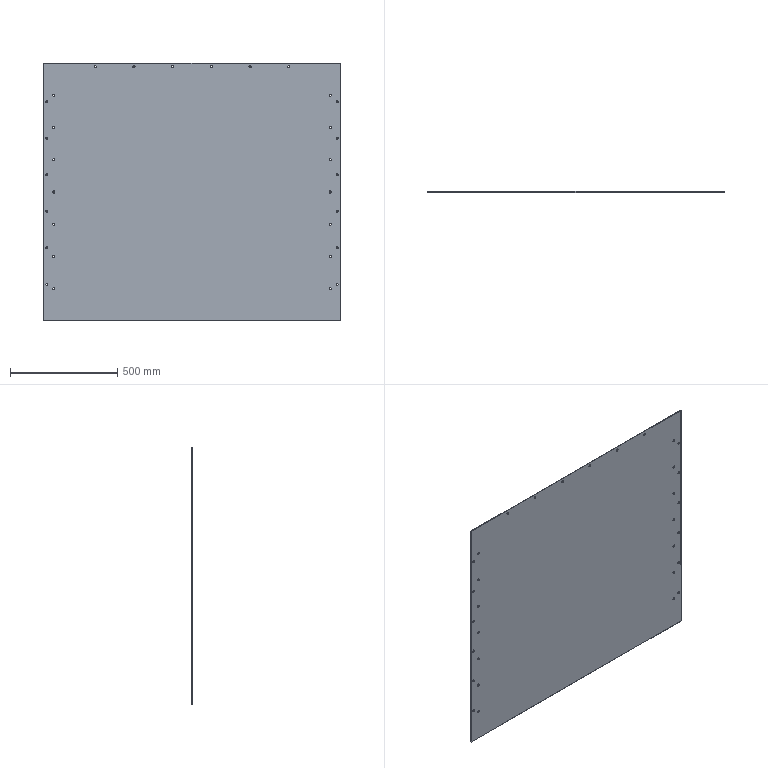Part | SolidWorks | features ICE 2, SMBaseFlange 2, FlatPattern 1, SheetMetal 1 | 1 solid | 70 faces | box 1380 x 3 x 1200 mm | volume 4960460 mm3 | cylinder 64 | plane 6 | commonest cylinder face diameters 10 x64